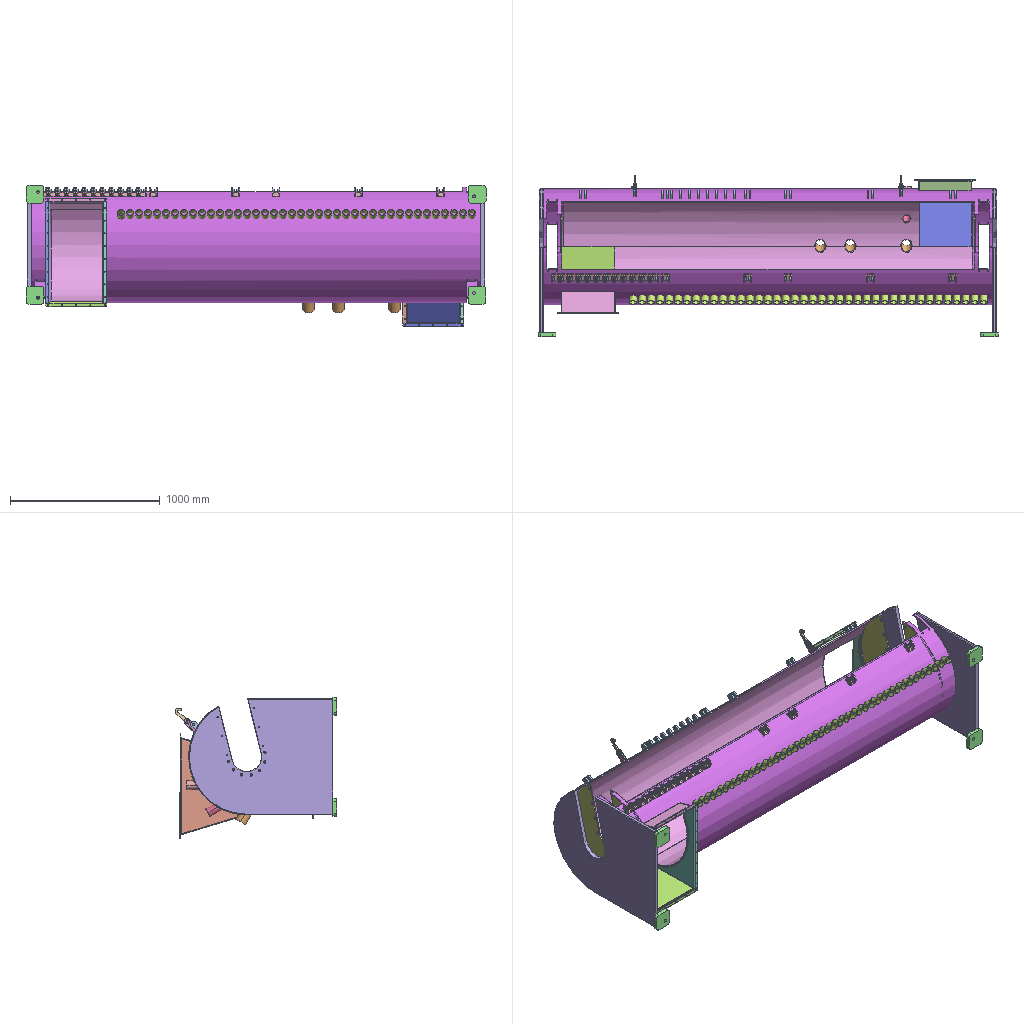Assembly | SolidWorks | 31 different items | 170 placed | box 3070 x 1077 x 944 mm
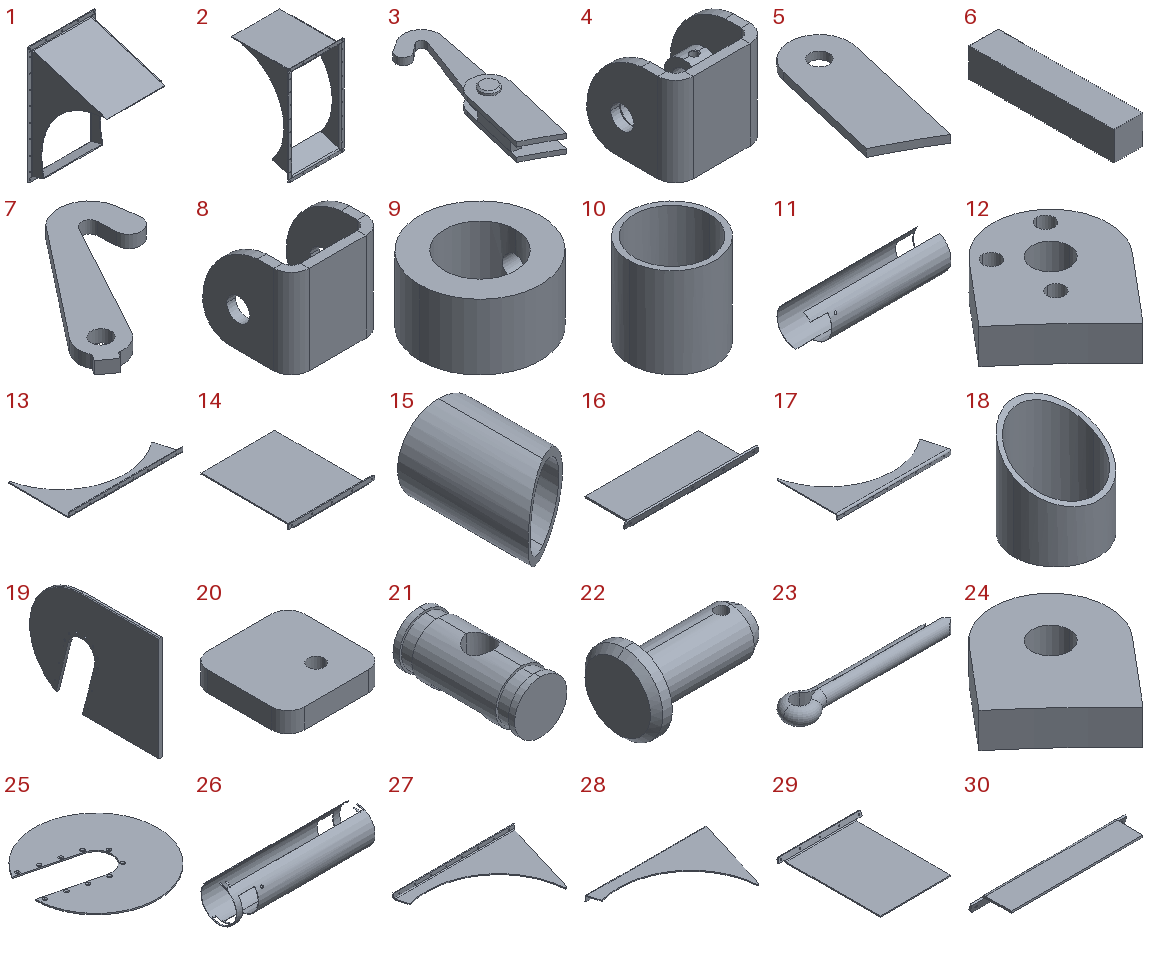Parts list (item | name | quantity | parent item | size | volume | features):
1 | (subassembly) | x1 | - | 405 x 446.049 x 700.825 mm | 2089258 mm3 | -
2 | (subassembly) | x1 | - | 410 x 445 x 723.639 mm | 2057835 mm3 | -
3 | (subassembly) | x2 | - | 67.815 x 194.526 x 32 mm | 74226 mm3 | features CompositeCurve 1
4 | (subassembly) | x17 | - | 52 x 50 x 50 mm | 35346 mm3 | -
5 | - | x4 | in 3 | 56.087 x 107.32 x 5 mm | 18280 mm3 | features Extrusion 1
6 | - | x4 | in 3 | 10 x 50 x 10 mm | 5000 mm3 | features Extrusion 1
7 | - | x2 | in 3 | 95.852 x 104.113 x 8 mm | 23315 mm3 | features Extrusion 1, Fillet 1
8 | - | x17 | in 4 | 52 x 50 x 50 mm | 29535 mm3 | features ICE 2, EdgeFlange 1, FlatPattern 1, SMBaseFlange 1, SheetMetal 1
9 | - | x34 | in 4 | 22 x 22 x 12 mm | 2905 mm3 | features 3DProfileFeature 1, Extrusion 1, HoleWzd 1
10 | - | x40 | - | 48.3 x 48.3 x 51.269 mm | 21706 mm3 | features Extrusion 1, ICE 1
11 | - | x1 | - | 2730 x 759 x 724.83 mm | 18223877 mm3 | features ICE 17, CirPattern 2, MirrorPattern 2, 3DProfileFeature 1, Extrusion 1, FlatPattern 1, FlattenBends 1, HoleWzd 1, ProcessBends 1, RefPoint 1, SheetMetal 1
12 | - | x1 | - | 53.274 x 55.837 x 12 mm | 18666 mm3 | features Extrusion 1, ICE 1
13 | - | x1 | in 2 | 673.852 x 361.966 x 30 mm | 462182 mm3 | features EdgeFlange 1, Fillet 1, FlatPattern 1, HoleWzd 1, LPattern 1, SMBaseFlange 1, SheetMetal 1
14 | - | x1 | in 2 | 410 x 445 x 30 mm | 821945 mm3 | features EdgeFlange 1, Fillet 1, FlatPattern 1, HoleWzd 1, LPattern 1, SMBaseFlange 1, SheetMetal 1
15 | - | x1 | - | 60 x 95.435 x 60 mm | 66487 mm3 | features Extrusion 1, ICE 1
16 | - | x1 | in 2 | 410 x 158.498 x 30.188 mm | 311527 mm3 | features 3DProfileFeature 1, EdgeFlange 1, Fillet 1, FlatPattern 1, HoleWzd 1, LPattern 1, SMBaseFlange 1, SheetMetal 1
17 | - | x1 | in 2 | 673.852 x 361.966 x 30 mm | 462182 mm3 | features 3DProfileFeature 1, EdgeFlange 1, Fillet 1, FlatPattern 1, HoleWzd 1, LPattern 1, SMBaseFlange 1, SheetMetal 1
18 | - | x3 | - | 76 x 76 x 85.679 mm | 57171 mm3 | features Extrusion 1, ICE 1
19 | - | x2 | - | 25 x 962.5 x 775 mm | 14615637 mm3 | features 3DProfileFeature 2, HoleWzd 2, Chamfer 1, CirPattern 1, Extrusion 1, ICE 1, LPattern 1, MirrorPattern 1
20 | - | x4 | - | 120 x 120 x 25 mm | 343562 mm3 | features Extrusion 1, Fillet 1
21 | - | x1 | - | 25 x 58 x 25 mm | 22422 mm3 | features ICE 3, Extrusion 1, MirrorPattern 1
22 | - | x2 | in 3 | 32 x 20 x 20 mm | 4166 mm3 | features MBimport 1
23 | - | x2 | in 3 | 29.6 x 5.8 x 2.9 mm | 185.002 mm3 | features ICE 1, Sweep 1
24 | - | x19 | - | 53.274 x 55.837 x 12 mm | 19684 mm3 | features Extrusion 1
25 | - | x2 | - | 758.937 x 759 x 8 mm | 2886950 mm3 | features Extrusion 1, HoleWzd 1
26 | - | x1 | - | 3000 x 775 x 774.928 mm | 40892506 mm3 | features ICE 10, MirrorPattern 2, 3DProfileFeature 1, CirPattern 1, Extrusion 1, FlatPattern 1, FlattenBends 1, HoleWzd 1, ProcessBends 1, RefPoint 1, SheetMetal 1
27 | - | x1 | in 1 | 651.256 x 419.882 x 30 mm | 529249 mm3 | features EdgeFlange 1, Fillet 1, FlatPattern 1, HoleWzd 1, LPattern 1, SMBaseFlange 1, SheetMetal 1
28 | - | x1 | in 1 | 651.256 x 419.882 x 30 mm | 531655 mm3 | features EdgeFlange 1, Fillet 1, FlatPattern 1, HoleWzd 1, LPattern 1, SMBaseFlange 1, SheetMetal 1
29 | - | x1 | in 1 | 405 x 473.792 x 30.148 mm | 850700 mm3 | features 3DProfileFeature 1, EdgeFlange 1, Fillet 1, FlatPattern 1, HoleWzd 1, SMBaseFlange 1, SheetMetal 1
30 | - | x1 | in 1 | 405 x 83.269 x 30.216 mm | 177655 mm3 | features EdgeFlange 1, Fillet 1, FlatPattern 1, HoleWzd 1, SMBaseFlange 1, SheetMetal 1
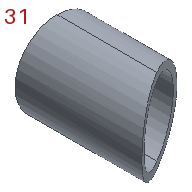31 | - | x1 | - | 60 x 90.775 x 60 mm | 62433 mm3 | features Extrusion 1, ICE 1
Mates (type | each side: item.copy, entity, surface, feature):
In the top assembly
Concentric | 7.1 face cylinder Boss-Extrude1 | 7.2 face cylinder Boss-Extrude1
Concentric | 31.1 select_type:24 | 26.1 face cylinder Round bend 1
Concentric | 13.1 face cylinder Base-Flange1 | 26.1 face cylinder Round bend 1
Coincident | 13.1 face plane Base-Flange1 | 26.1 face plane Round bend 1
Parallel | 16.1 face plane Edge-Flange1 | 19.1 face plane Boss-Extrude1
Coincident | 18.1 face plane Boss-Extrude1 | 18.2 face plane Boss-Extrude1
Coincident | 26.1 select_type:24 | 18.1 plane
Concentric | 26.1 select_type:24 | 18.1 face cylinder Boss-Extrude1
DistanceDim | 26.1 plane | 18.1 face plane Boss-Extrude1
Coincident | 18.2 face plane Boss-Extrude1 | 18.3 face plane Boss-Extrude1
Coincident | 18.2 plane | 18.3 plane
Concentric | 26.1 select_type:24 | 18.2 face cylinder Boss-Extrude1
Concentric | 26.1 select_type:24 | 18.3 face cylinder Boss-Extrude1
Concentric | 26.1 face cylinder Round bend 1 | 19.1 face cylinder Boss-Extrude1
Coincident | 26.1 face plane Round bend 1 | 19.1 face plane Boss-Extrude1
Parallel | 25.1 face plane Boss-Extrude1 | 19.1 face plane Cut-Extrude1
Coincident | 20.1 face plane Boss-Extrude1 | 20.2 face plane Boss-Extrude1
Coincident | 26.1 plane | 15.1 plane
Concentric | 26.1 select_type:24 | 15.1 face cylinder Boss-Extrude1
Coincident | 26.1 face cylinder Round bend 1 | 15.1 select_type:25
Concentric | 24.1 face cylinder Boss-Extrude1 | 26.1 face cylinder Round bend 1
PlanarAngleDim | 26.1 plane | 24.1 face plane Boss-Extrude1
Concentric | 26.1 face cylinder Round bend 1 | 24.1 face cylinder Boss-Extrude1
Concentric | 26.1 face cylinder Round bend 1 | 25.1 face cylinder Boss-Extrude1
Coincident | 26.1 face plane Round bend 1 | 25.1 face plane Boss-Extrude1
Parallel | 13.1 face plane Edge-Flange1 | assembly plane
Concentric | 5.1 face cylinder Boss-Extrude1 | 26.1 face cylinder Round bend 1
Concentric | 26.1 face cylinder Round bend 1 | 5.2 face cylinder Boss-Extrude1
Concentric | 5.3 face cylinder Boss-Extrude1 | 26.1 face cylinder Round bend 1
DistanceDim | 26.1 edge | 5.4 face plane Boss-Extrude1
Tangent | 26.1 face cylinder Round bend 1 | 8.1 face plane Base-Flange1
DistanceDim | 8.1 edge | 26.1 face plane Round bend 1
Coincident | 26.1 face cylinder Round bend 1 | 8.1 edge
Coincident | 26.1 face cylinder Round bend 1 | 8.2 edge
Tangent | 26.1 face cylinder Round bend 1 | 8.2 face plane Base-Flange1
DistanceDim | 8.2 edge | 26.1 face plane Round bend 1
Concentric | 28.1 face cylinder Base-Flange1 | 26.1 face cylinder Round bend 1
Coincident | 27.1 face plane Base-Flange1 | 26.1 face plane Round bend 1
Coincident | 29.1 edge | 26.1 face plane Round bend 1
Concentric | 26.1 face cylinder Round bend 1 | 25.2 face cylinder Boss-Extrude1
Parallel | 19.2 face plane Cut-Extrude1 | 25.2 face plane Boss-Extrude1
Coincident | 26.1 face plane Round bend 1 | 25.2 face plane Boss-Extrude1
Concentric | 24.2 face cylinder Boss-Extrude1 | 26.1 face cylinder Round bend 1
DistanceDim | 24.3 face plane Boss-Extrude1 | 26.1 face plane Round bend 1
DistanceDim | 26.1 face plane Round bend 1 | 24.3 edge
DistanceDim | 5.3 face plane Boss-Extrude1 | 26.1 face plane Round bend 1
DistanceDim | 5.2 face plane Boss-Extrude1 | 26.1 face plane Round bend 1
DistanceDim | 24.3 face plane Boss-Extrude1 | 4.1 plane
DistanceDim | 24.1 face plane Boss-Extrude1 | 26.1 face plane Round bend 1
DistanceDim | 4.2 plane | 24.4 face plane Boss-Extrude1
Concentric | 26.1 select_type:24 | 10.1 face cylinder Boss-Extrude1
Coincident | 26.1 face cylinder Round bend 1 | 10.1 select_type:24
Coincident | 26.1 plane | 11.1 plane | 2 times
Concentric | 26.1 face cylinder Round bend 1 | 12.1 face cylinder Boss-Extrude1
Coincident | 24.5 edge | 12.1 edge
DistanceDim | 12.1 face plane Boss-Extrude1 | 24.5 face plane Boss-Extrude1
Concentric | 26.1 face cylinder Round bend 1 | 11.1 face cylinder Round bend 3
Coincident | 26.1 plane | assembly plane
DistanceDim | 19.2 face plane Boss-Extrude1 | 20.1 face plane Boss-Extrude1 | 2 times
Coincident | 20.1 face plane Boss-Extrude1 | 19.2 face plane Boss-Extrude1
Concentric | 31.1 face cylinder Boss-Extrude1 | 26.1 select_type:24
In subassembly 4
Coincident | 8.3 plane | 4.3 plane | 3 times
Concentric | 8.3 face cylinder Cut-Extrude1 | 4.3 face
DistanceDim | 4.3 face | 8.3 face plane Edge-Flange1
Coincident | 4.3 face | 4.3 face
In subassembly 3
Coincident | 5.5 plane | 3.1 plane | 3 times
Coincident | 5.5 face plane Boss-Extrude1 | 6.1 face plane Boss-Extrude1 | 2 times
DistanceDim | 5.5 edge | 6.1 face plane Boss-Extrude1
Coincident | 5.5 face plane Boss-Extrude1 | 6.2 face plane Boss-Extrude1 | 2 times
Coincident | 6.1 face plane Boss-Extrude1 | 6.2 face plane Boss-Extrude1
Coincident | 6.2 face plane Boss-Extrude1 | 5.6 face plane Boss-Extrude1
Coincident | 5.5 face plane Boss-Extrude1 | 5.6 face plane Boss-Extrude1
Concentric | 5.5 face cylinder Boss-Extrude1 | 5.6 face cylinder Boss-Extrude1
Coincident | 6.2 plane | 7.3 plane
Concentric | 5.6 face cylinder Boss-Extrude1 | 7.3 face cylinder Boss-Extrude1
Concentric | 7.3 face cylinder Boss-Extrude1 | 22.1 face cylinder GB╱T 882-2008[clevis pin type B 12×28].step<1>
Coincident | 5.5 face plane Boss-Extrude1 | 22.1 face plane GB╱T 882-2008[clevis pin type B 12×28].step<1>
Concentric | 22.1 face cylinder GB╱T 882-2008[clevis pin type B 12×28].step<1> | 23.1 face cylinder Sweep2
Tangent | 22.1 face cylinder GB╱T 882-2008[clevis pin type B 12×28].step<1> | 23.1 edge
In subassembly 1
DistanceDim | 27.2 face plane Base-Flange1 | 1.1 plane
DistanceDim | 28.2 face plane Base-Flange1 | 1.1 plane
Coincident | 27.2 plane | 1.1 plane | 2 times
Coincident | 28.2 plane | 1.1 plane | 2 times
Coincident | 29.2 plane | 1.1 plane
Coincident | 30.1 plane | 1.1 plane
Coincident | 28.2 face plane Base-Flange1 | 30.1 face plane Base-Flange1
Coincident | 27.2 face plane Base-Flange1 | 29.2 face plane Base-Flange1
Coincident | 27.2 face plane Edge-Flange1 | 29.2 face plane Edge-Flange1
Coincident | 27.2 face plane Edge-Flange1 | 30.1 face plane Edge-Flange1
In subassembly 2
DistanceDim | 13.2 face plane Base-Flange1 | 2.1 plane
DistanceDim | 17.1 face plane Base-Flange1 | 2.1 plane
Coincident | 13.2 plane | 2.1 plane
Coincident | 13.2 face plane Edge-Flange1 | 2.1 plane
Concentric | 13.2 face cylinder Base-Flange1 | 17.1 face cylinder Base-Flange1
Coincident | 13.2 face plane Edge-Flange1 | 17.1 face plane Edge-Flange1
Coincident | 14.1 plane | 2.1 plane
Coincident | 16.2 plane | 2.1 plane
Coincident | 16.2 face plane Base-Flange1 | 17.1 face plane Base-Flange1
Coincident | 14.1 face plane Base-Flange1 | 17.1 face plane Base-Flange1
Coincident | 16.2 face plane Edge-Flange1 | 17.1 face plane Edge-Flange1
Coincident | 14.1 face plane Edge-Flange1 | 17.1 face plane Edge-Flange1